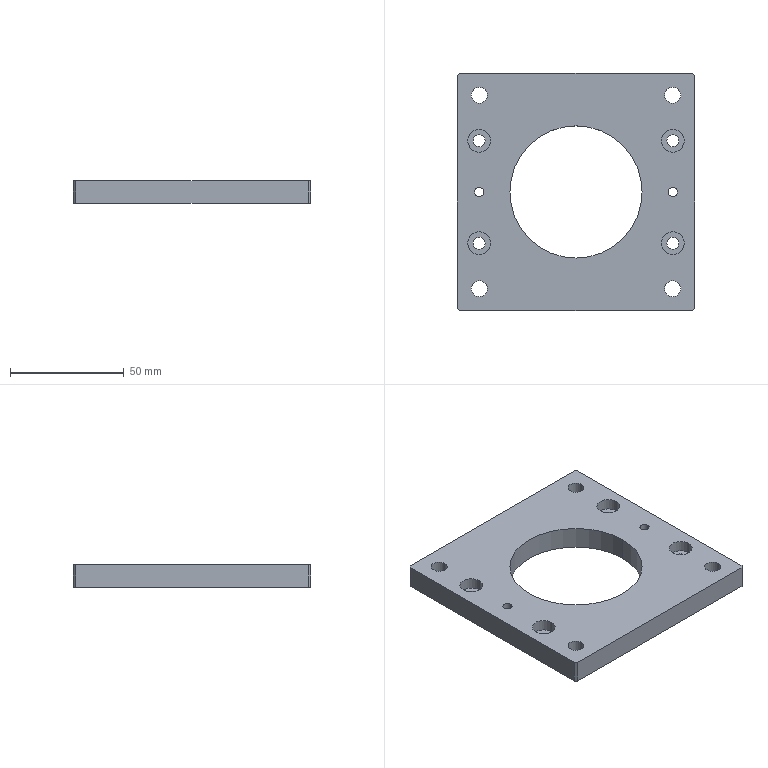Part | STEP file | CON-010 | 1 solid | 44 faces | box 104 x 104 x 10 mm | volume 77916 mm3 | cylinder 30 | plane 14 | commonest cylinder face diameters 5.3 x8 7 x8 10 x8 4 x4 58 x2